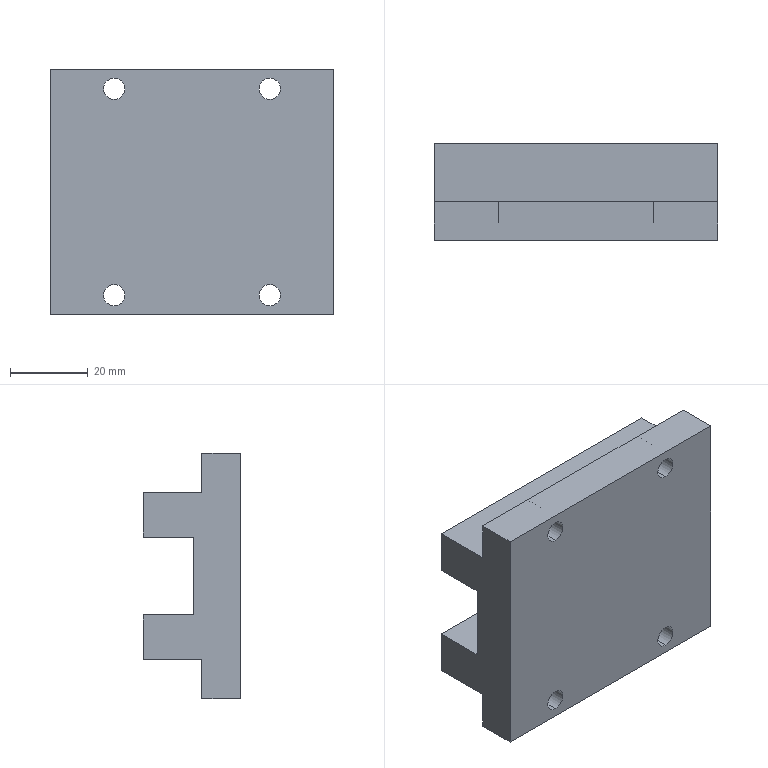Part | STEP file | copy of MSA20EA.stp^PN_0017_default | 1 solid | 34 faces | box 72.9 x 25 x 63 mm | volume 72025 mm3 | plane 18 | cylinder 16 | commonest cylinder face diameters 5.5 x8 9.5 x8